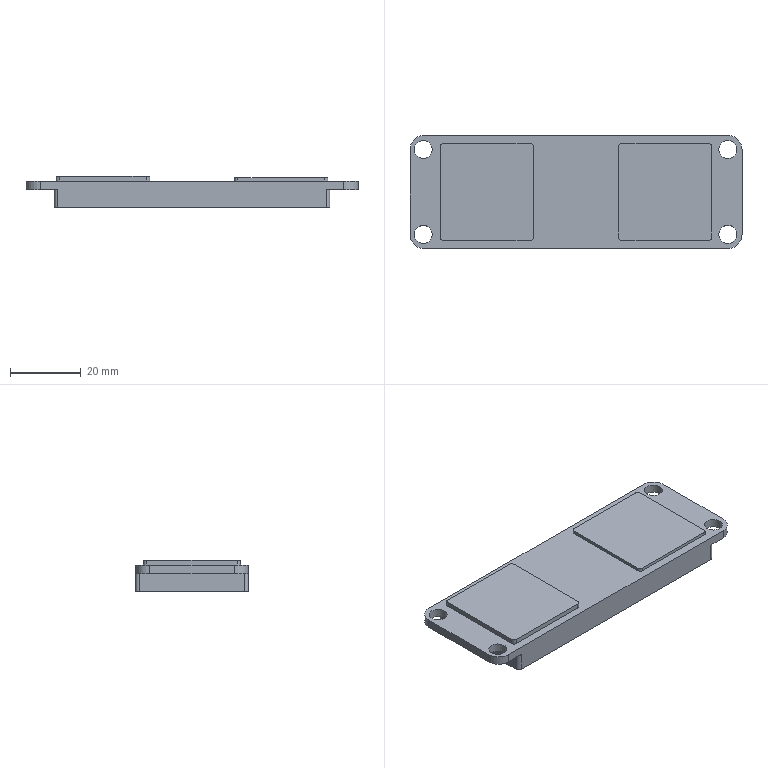Part | 1 solid | 101 faces | box 94 x 32 x 9 mm | volume 17484 mm3 | cylinder 46 | plane 35 | cone 12 | torus 8 | commonest cylinder face diameters 2 x12 0.6 x8 2.5 x6 5.1 x4 8 x4 5.5 x2